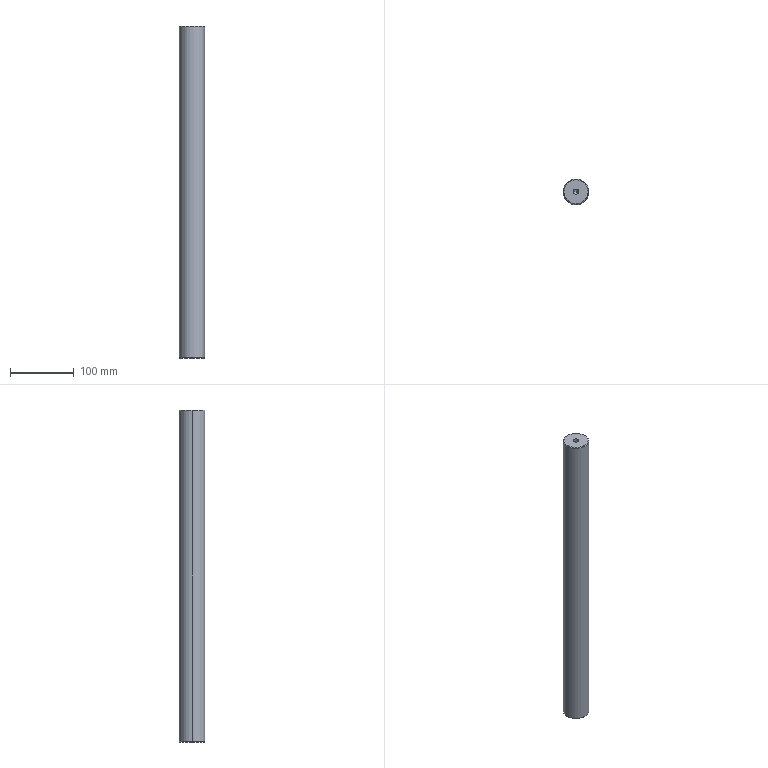Part | SolidWorks | features Chamfer 2, HoleWzd 2, Extrusion 1 | 1 solid | 16 faces | box 40 x 40 x 520 mm | volume 650025 mm3 | cone 8 | cylinder 6 | plane 2 | commonest cylinder face diameters 8.5 x4 40 x2
STEP:
#1=CARTESIAN_POINT('',(-4.25,0.,495.5));
#2=VERTEX_POINT('',#1);
#3=CARTESIAN_POINT('',(4.25,0.,495.5));
#4=VERTEX_POINT('',#3);
#5=CARTESIAN_POINT('',(0.,0.,495.5));
#6=DIRECTION('',(0.,0.,1.));
#7=DIRECTION('',(1.,0.,0.));
#8=AXIS2_PLACEMENT_3D('',#5,#6,#7);
#9=CIRCLE('',#8,4.25);
#10=EDGE_CURVE('',#2,#4,#9,.T.);
#11=ORIENTED_EDGE('',*,*,#10,.F.);
#12=CARTESIAN_POINT('',(-4.25,0.,520.));
#13=VERTEX_POINT('',#12);
#14=CARTESIAN_POINT('',(-4.25,0.,520.));
#15=DIRECTION('',(0.,0.,1.));
#16=VECTOR('',#15,1000.);
#17=LINE('',#14,#16);
#18=EDGE_CURVE('',#2,#13,#17,.T.);
#19=ORIENTED_EDGE('',*,*,#18,.T.);
#20=CARTESIAN_POINT('',(4.25,0.,520.));
#21=VERTEX_POINT('',#20);
#22=CARTESIAN_POINT('',(0.,0.,520.));
#23=DIRECTION('',(0.,0.,1.));
#24=DIRECTION('',(1.,0.,0.));
#25=AXIS2_PLACEMENT_3D('',#22,#23,#24);
#26=CIRCLE('',#25,4.25);
#27=EDGE_CURVE('',#13,#21,#26,.T.);
#28=ORIENTED_EDGE('',*,*,#27,.T.);
#29=CARTESIAN_POINT('',(4.25,0.,520.));
#30=DIRECTION('',(0.,0.,1.));
#31=VECTOR('',#30,1000.);
#32=LINE('',#29,#31);
#33=EDGE_CURVE('',#4,#21,#32,.T.);
#34=ORIENTED_EDGE('',*,*,#33,.F.);
#35=EDGE_LOOP('',(#11,#19,#28,#34));
#36=FACE_OUTER_BOUND('',#35,.T.);
#37=CARTESIAN_POINT('',(0.,0.,520.));
#38=DIRECTION('',(0.,0.,1.));
#39=DIRECTION('',(1.,0.,0.));
#40=AXIS2_PLACEMENT_3D('',#37,#38,#39);
#41=CYLINDRICAL_SURFACE('',#40,4.25);
#42=ADVANCED_FACE('',(#36),#41,.F.);
#43=CARTESIAN_POINT('',(0.,0.,492.946));
#44=VERTEX_POINT('',#43);
#45=CARTESIAN_POINT('',(4.25,0.,495.5));
#46=DIRECTION('',(0.8572,0.,0.515));
#47=VECTOR('',#46,1000.);
#48=LINE('',#45,#47);
#49=EDGE_CURVE('',#44,#4,#48,.T.);
#50=ORIENTED_EDGE('',*,*,#49,.F.);
#51=CARTESIAN_POINT('',(-4.25,0.,495.5));
#52=DIRECTION('',(-0.8572,0.,0.515));
#53=VECTOR('',#52,1000.);
#54=LINE('',#51,#53);
#55=EDGE_CURVE('',#44,#2,#54,.T.);
#56=ORIENTED_EDGE('',*,*,#55,.T.);
#57=ORIENTED_EDGE('',*,*,#10,.T.);
#58=EDGE_LOOP('',(#50,#56,#57));
#59=FACE_OUTER_BOUND('',#58,.T.);
#60=CARTESIAN_POINT('',(0.,0.,495.5));
#61=DIRECTION('',(0.,0.,1.));
#62=DIRECTION('',(1.,0.,0.));
#63=AXIS2_PLACEMENT_3D('',#60,#61,#62);
#64=CONICAL_SURFACE('',#63,4.25,1.03);
#65=ADVANCED_FACE('',(#59),#64,.F.);
#66=CARTESIAN_POINT('',(-19.,0.,0.));
#67=VERTEX_POINT('',#66);
#68=CARTESIAN_POINT('',(19.,0.,0.));
#69=VERTEX_POINT('',#68);
#70=CARTESIAN_POINT('',(0.,0.,0.));
#71=DIRECTION('',(0.,0.,-1.));
#72=DIRECTION('',(1.,0.,0.));
#73=AXIS2_PLACEMENT_3D('',#70,#71,#72);
#74=CIRCLE('',#73,19.);
#75=EDGE_CURVE('',#67,#69,#74,.T.);
#76=ORIENTED_EDGE('',*,*,#75,.F.);
#77=CARTESIAN_POINT('',(-20.,0.,1.));
#78=VERTEX_POINT('',#77);
#79=CARTESIAN_POINT('',(-20.,0.,1.));
#80=DIRECTION('',(-0.7071,0.,0.7071));
#81=VECTOR('',#80,1000.);
#82=LINE('',#79,#81);
#83=EDGE_CURVE('',#67,#78,#82,.T.);
#84=ORIENTED_EDGE('',*,*,#83,.T.);
#85=CARTESIAN_POINT('',(20.,0.,1.));
#86=VERTEX_POINT('',#85);
#87=CARTESIAN_POINT('',(0.,0.,1.));
#88=DIRECTION('',(0.,0.,1.));
#89=DIRECTION('',(1.,0.,0.));
#90=AXIS2_PLACEMENT_3D('',#87,#88,#89);
#91=CIRCLE('',#90,20.);
#92=EDGE_CURVE('',#86,#78,#91,.T.);
#93=ORIENTED_EDGE('',*,*,#92,.F.);
#94=CARTESIAN_POINT('',(20.,0.,1.));
#95=DIRECTION('',(0.7071,0.,0.7071));
#96=VECTOR('',#95,1000.);
#97=LINE('',#94,#96);
#98=EDGE_CURVE('',#69,#86,#97,.T.);
#99=ORIENTED_EDGE('',*,*,#98,.F.);
#100=EDGE_LOOP('',(#76,#84,#93,#99));
#101=FACE_OUTER_BOUND('',#100,.T.);
#102=CARTESIAN_POINT('',(0.,0.,1.));
#103=DIRECTION('',(0.,0.,1.));
#104=DIRECTION('',(1.,0.,0.));
#105=AXIS2_PLACEMENT_3D('',#102,#103,#104);
#106=CONICAL_SURFACE('',#105,20.,0.7854);
#107=ADVANCED_FACE('',(#101),#106,.T.);
#108=CARTESIAN_POINT('',(19.,0.,520.));
#109=VERTEX_POINT('',#108);
#110=CARTESIAN_POINT('',(-19.,0.,520.));
#111=VERTEX_POINT('',#110);
#112=CARTESIAN_POINT('',(0.,0.,520.));
#113=DIRECTION('',(0.,0.,1.));
#114=DIRECTION('',(1.,0.,0.));
#115=AXIS2_PLACEMENT_3D('',#112,#113,#114);
#116=CIRCLE('',#115,19.);
#117=EDGE_CURVE('',#109,#111,#116,.T.);
#118=ORIENTED_EDGE('',*,*,#117,.F.);
#119=CARTESIAN_POINT('',(20.,0.,519.));
#120=VERTEX_POINT('',#119);
#121=CARTESIAN_POINT('',(19.,0.,520.));
#122=DIRECTION('',(0.7071,0.,-0.7071));
#123=VECTOR('',#122,1000.);
#124=LINE('',#121,#123);
#125=EDGE_CURVE('',#109,#120,#124,.T.);
#126=ORIENTED_EDGE('',*,*,#125,.T.);
#127=CARTESIAN_POINT('',(-20.,0.,519.));
#128=VERTEX_POINT('',#127);
#129=CARTESIAN_POINT('',(0.,0.,519.));
#130=DIRECTION('',(0.,0.,-1.));
#131=DIRECTION('',(1.,0.,0.));
#132=AXIS2_PLACEMENT_3D('',#129,#130,#131);
#133=CIRCLE('',#132,20.);
#134=EDGE_CURVE('',#128,#120,#133,.T.);
#135=ORIENTED_EDGE('',*,*,#134,.F.);
#136=CARTESIAN_POINT('',(-19.,0.,520.));
#137=DIRECTION('',(-0.7071,0.,-0.7071));
#138=VECTOR('',#137,1000.);
#139=LINE('',#136,#138);
#140=EDGE_CURVE('',#111,#128,#139,.T.);
#141=ORIENTED_EDGE('',*,*,#140,.F.);
#142=EDGE_LOOP('',(#118,#126,#135,#141));
#143=FACE_OUTER_BOUND('',#142,.T.);
#144=CARTESIAN_POINT('',(0.,0.,520.));
#145=DIRECTION('',(0.,0.,-1.));
#146=DIRECTION('',(-1.,0.,0.));
#147=AXIS2_PLACEMENT_3D('',#144,#145,#146);
#148=CONICAL_SURFACE('',#147,19.,0.7854);
#149=ADVANCED_FACE('',(#143),#148,.T.);
#150=CARTESIAN_POINT('',(4.25,0.,32.));
#151=VERTEX_POINT('',#150);
#152=CARTESIAN_POINT('',(-4.25,0.,32.));
#153=VERTEX_POINT('',#152);
#154=CARTESIAN_POINT('',(0.,0.,32.));
#155=DIRECTION('',(0.,0.,-1.));
#156=DIRECTION('',(-1.,0.,0.));
#157=AXIS2_PLACEMENT_3D('',#154,#155,#156);
#158=CIRCLE('',#157,4.25);
#159=EDGE_CURVE('',#151,#153,#158,.T.);
#160=ORIENTED_EDGE('',*,*,#159,.F.);
#161=CARTESIAN_POINT('',(4.25,0.,0.));
#162=VERTEX_POINT('',#161);
#163=CARTESIAN_POINT('',(4.25,0.,0.));
#164=DIRECTION('',(0.,0.,-1.));
#165=VECTOR('',#164,1000.);
#166=LINE('',#163,#165);
#167=EDGE_CURVE('',#151,#162,#166,.T.);
#168=ORIENTED_EDGE('',*,*,#167,.T.);
#169=CARTESIAN_POINT('',(-4.25,0.,0.));
#170=VERTEX_POINT('',#169);
#171=CARTESIAN_POINT('',(0.,0.,0.));
#172=DIRECTION('',(0.,0.,-1.));
#173=DIRECTION('',(-1.,0.,0.));
#174=AXIS2_PLACEMENT_3D('',#171,#172,#173);
#175=CIRCLE('',#174,4.25);
#176=EDGE_CURVE('',#162,#170,#175,.T.);
#177=ORIENTED_EDGE('',*,*,#176,.T.);
#178=CARTESIAN_POINT('',(-4.25,0.,0.));
#179=DIRECTION('',(0.,0.,-1.));
#180=VECTOR('',#179,1000.);
#181=LINE('',#178,#180);
#182=EDGE_CURVE('',#153,#170,#181,.T.);
#183=ORIENTED_EDGE('',*,*,#182,.F.);
#184=EDGE_LOOP('',(#160,#168,#177,#183));
#185=FACE_OUTER_BOUND('',#184,.T.);
#186=CARTESIAN_POINT('',(0.,0.,0.));
#187=DIRECTION('',(0.,0.,-1.));
#188=DIRECTION('',(-1.,0.,0.));
#189=AXIS2_PLACEMENT_3D('',#186,#187,#188);
#190=CYLINDRICAL_SURFACE('',#189,4.25);
#191=ADVANCED_FACE('',(#185),#190,.F.);
#192=CARTESIAN_POINT('',(0.,0.,34.554));
#193=VERTEX_POINT('',#192);
#194=CARTESIAN_POINT('',(-4.25,0.,32.));
#195=DIRECTION('',(-0.8572,0.,-0.515));
#196=VECTOR('',#195,1000.);
#197=LINE('',#194,#196);
#198=EDGE_CURVE('',#193,#153,#197,.T.);
#199=ORIENTED_EDGE('',*,*,#198,.F.);
#200=CARTESIAN_POINT('',(4.25,0.,32.));
#201=DIRECTION('',(0.8572,0.,-0.515));
#202=VECTOR('',#201,1000.);
#203=LINE('',#200,#202);
#204=EDGE_CURVE('',#193,#151,#203,.T.);
#205=ORIENTED_EDGE('',*,*,#204,.T.);
#206=ORIENTED_EDGE('',*,*,#159,.T.);
#207=EDGE_LOOP('',(#199,#205,#206));
#208=FACE_OUTER_BOUND('',#207,.T.);
#209=CARTESIAN_POINT('',(0.,0.,32.));
#210=DIRECTION('',(0.,0.,-1.));
#211=DIRECTION('',(-1.,0.,0.));
#212=AXIS2_PLACEMENT_3D('',#209,#210,#211);
#213=CONICAL_SURFACE('',#212,4.25,1.03);
#214=ADVANCED_FACE('',(#208),#213,.F.);
#215=ORIENTED_EDGE('',*,*,#134,.T.);
#216=CARTESIAN_POINT('',(20.,0.,520.));
#217=DIRECTION('',(0.,0.,-1.));
#218=VECTOR('',#217,1000.);
#219=LINE('',#216,#218);
#220=EDGE_CURVE('',#120,#86,#219,.T.);
#221=ORIENTED_EDGE('',*,*,#220,.T.);
#222=ORIENTED_EDGE('',*,*,#92,.T.);
#223=CARTESIAN_POINT('',(-20.,0.,520.));
#224=DIRECTION('',(0.,0.,-1.));
#225=VECTOR('',#224,1000.);
#226=LINE('',#223,#225);
#227=EDGE_CURVE('',#128,#78,#226,.T.);
#228=ORIENTED_EDGE('',*,*,#227,.F.);
#229=EDGE_LOOP('',(#215,#221,#222,#228));
#230=FACE_OUTER_BOUND('',#229,.T.);
#231=CARTESIAN_POINT('',(0.,0.,520.));
#232=DIRECTION('',(0.,0.,-1.));
#233=DIRECTION('',(-1.,0.,0.));
#234=AXIS2_PLACEMENT_3D('',#231,#232,#233);
#235=CYLINDRICAL_SURFACE('',#234,20.);
#236=ADVANCED_FACE('',(#230),#235,.T.);
#237=ORIENTED_EDGE('',*,*,#220,.F.);
#238=CARTESIAN_POINT('',(0.,0.,519.));
#239=DIRECTION('',(0.,0.,-1.));
#240=DIRECTION('',(1.,0.,0.));
#241=AXIS2_PLACEMENT_3D('',#238,#239,#240);
#242=CIRCLE('',#241,20.);
#243=EDGE_CURVE('',#120,#128,#242,.T.);
#244=ORIENTED_EDGE('',*,*,#243,.T.);
#245=ORIENTED_EDGE('',*,*,#227,.T.);
#246=CARTESIAN_POINT('',(0.,0.,1.));
#247=DIRECTION('',(0.,0.,1.));
#248=DIRECTION('',(1.,0.,0.));
#249=AXIS2_PLACEMENT_3D('',#246,#247,#248);
#250=CIRCLE('',#249,20.);
#251=EDGE_CURVE('',#78,#86,#250,.T.);
#252=ORIENTED_EDGE('',*,*,#251,.T.);
#253=EDGE_LOOP('',(#237,#244,#245,#252));
#254=FACE_OUTER_BOUND('',#253,.T.);
#255=CARTESIAN_POINT('',(0.,0.,520.));
#256=DIRECTION('',(0.,0.,-1.));
#257=DIRECTION('',(-1.,0.,0.));
#258=AXIS2_PLACEMENT_3D('',#255,#256,#257);
#259=CYLINDRICAL_SURFACE('',#258,20.);
#260=ADVANCED_FACE('',(#254),#259,.T.);
#261=CARTESIAN_POINT('',(0.,0.,520.));
#262=DIRECTION('',(0.,0.,1.));
#263=DIRECTION('',(1.,0.,0.));
#264=AXIS2_PLACEMENT_3D('',#261,#262,#263);
#265=CIRCLE('',#264,4.25);
#266=EDGE_CURVE('',#21,#13,#265,.T.);
#267=ORIENTED_EDGE('',*,*,#266,.F.);
#268=ORIENTED_EDGE('',*,*,#27,.F.);
#269=EDGE_LOOP('',(#267,#268));
#270=FACE_BOUND('',#269,.T.);
#271=CARTESIAN_POINT('',(0.,0.,520.));
#272=DIRECTION('',(0.,0.,1.));
#273=DIRECTION('',(1.,0.,0.));
#274=AXIS2_PLACEMENT_3D('',#271,#272,#273);
#275=CIRCLE('',#274,19.);
#276=EDGE_CURVE('',#111,#109,#275,.T.);
#277=ORIENTED_EDGE('',*,*,#276,.T.);
#278=ORIENTED_EDGE('',*,*,#117,.T.);
#279=EDGE_LOOP('',(#277,#278));
#280=FACE_OUTER_BOUND('',#279,.T.);
#281=CARTESIAN_POINT('',(0.,0.,520.));
#282=DIRECTION('',(0.,0.,1.));
#283=DIRECTION('',(1.,0.,0.));
#284=AXIS2_PLACEMENT_3D('',#281,#282,#283);
#285=PLANE('',#284);
#286=ADVANCED_FACE('',(#270,#280),#285,.T.);
#287=CARTESIAN_POINT('',(0.,0.,0.));
#288=DIRECTION('',(0.,0.,-1.));
#289=DIRECTION('',(1.,0.,0.));
#290=AXIS2_PLACEMENT_3D('',#287,#288,#289);
#291=CIRCLE('',#290,19.);
#292=EDGE_CURVE('',#69,#67,#291,.T.);
#293=ORIENTED_EDGE('',*,*,#292,.T.);
#294=ORIENTED_EDGE('',*,*,#75,.T.);
#295=EDGE_LOOP('',(#293,#294));
#296=FACE_OUTER_BOUND('',#295,.T.);
#297=CARTESIAN_POINT('',(0.,0.,0.));
#298=DIRECTION('',(0.,0.,-1.));
#299=DIRECTION('',(-1.,0.,0.));
#300=AXIS2_PLACEMENT_3D('',#297,#298,#299);
#301=CIRCLE('',#300,4.25);
#302=EDGE_CURVE('',#170,#162,#301,.T.);
#303=ORIENTED_EDGE('',*,*,#302,.F.);
#304=ORIENTED_EDGE('',*,*,#176,.F.);
#305=EDGE_LOOP('',(#303,#304));
#306=FACE_BOUND('',#305,.T.);
#307=CARTESIAN_POINT('',(0.,0.,0.));
#308=DIRECTION('',(0.,0.,1.));
#309=DIRECTION('',(1.,0.,0.));
#310=AXIS2_PLACEMENT_3D('',#307,#308,#309);
#311=PLANE('',#310);
#312=ADVANCED_FACE('',(#296,#306),#311,.F.);
#313=ORIENTED_EDGE('',*,*,#204,.F.);
#314=ORIENTED_EDGE('',*,*,#198,.T.);
#315=CARTESIAN_POINT('',(0.,0.,32.));
#316=DIRECTION('',(0.,0.,-1.));
#317=DIRECTION('',(-1.,0.,0.));
#318=AXIS2_PLACEMENT_3D('',#315,#316,#317);
#319=CIRCLE('',#318,4.25);
#320=EDGE_CURVE('',#153,#151,#319,.T.);
#321=ORIENTED_EDGE('',*,*,#320,.T.);
#322=EDGE_LOOP('',(#313,#314,#321));
#323=FACE_OUTER_BOUND('',#322,.T.);
#324=CARTESIAN_POINT('',(0.,0.,32.));
#325=DIRECTION('',(0.,0.,-1.));
#326=DIRECTION('',(-1.,0.,0.));
#327=AXIS2_PLACEMENT_3D('',#324,#325,#326);
#328=CONICAL_SURFACE('',#327,4.25,1.03);
#329=ADVANCED_FACE('',(#323),#328,.F.);
#330=ORIENTED_EDGE('',*,*,#167,.F.);
#331=ORIENTED_EDGE('',*,*,#320,.F.);
#332=ORIENTED_EDGE('',*,*,#182,.T.);
#333=ORIENTED_EDGE('',*,*,#302,.T.);
#334=EDGE_LOOP('',(#330,#331,#332,#333));
#335=FACE_OUTER_BOUND('',#334,.T.);
#336=CARTESIAN_POINT('',(0.,0.,0.));
#337=DIRECTION('',(0.,0.,-1.));
#338=DIRECTION('',(-1.,0.,0.));
#339=AXIS2_PLACEMENT_3D('',#336,#337,#338);
#340=CYLINDRICAL_SURFACE('',#339,4.25);
#341=ADVANCED_FACE('',(#335),#340,.F.);
#342=ORIENTED_EDGE('',*,*,#125,.F.);
#343=ORIENTED_EDGE('',*,*,#276,.F.);
#344=ORIENTED_EDGE('',*,*,#140,.T.);
#345=ORIENTED_EDGE('',*,*,#243,.F.);
#346=EDGE_LOOP('',(#342,#343,#344,#345));
#347=FACE_OUTER_BOUND('',#346,.T.);
#348=CARTESIAN_POINT('',(0.,0.,520.));
#349=DIRECTION('',(0.,0.,-1.));
#350=DIRECTION('',(-1.,0.,0.));
#351=AXIS2_PLACEMENT_3D('',#348,#349,#350);
#352=CONICAL_SURFACE('',#351,19.,0.7854);
#353=ADVANCED_FACE('',(#347),#352,.T.);
#354=ORIENTED_EDGE('',*,*,#83,.F.);
#355=ORIENTED_EDGE('',*,*,#292,.F.);
#356=ORIENTED_EDGE('',*,*,#98,.T.);
#357=ORIENTED_EDGE('',*,*,#251,.F.);
#358=EDGE_LOOP('',(#354,#355,#356,#357));
#359=FACE_OUTER_BOUND('',#358,.T.);
#360=CARTESIAN_POINT('',(0.,0.,1.));
#361=DIRECTION('',(0.,0.,1.));
#362=DIRECTION('',(1.,0.,0.));
#363=AXIS2_PLACEMENT_3D('',#360,#361,#362);
#364=CONICAL_SURFACE('',#363,20.,0.7854);
#365=ADVANCED_FACE('',(#359),#364,.T.);
#366=ORIENTED_EDGE('',*,*,#55,.F.);
#367=ORIENTED_EDGE('',*,*,#49,.T.);
#368=CARTESIAN_POINT('',(0.,0.,495.5));
#369=DIRECTION('',(0.,0.,1.));
#370=DIRECTION('',(1.,0.,0.));
#371=AXIS2_PLACEMENT_3D('',#368,#369,#370);
#372=CIRCLE('',#371,4.25);
#373=EDGE_CURVE('',#4,#2,#372,.T.);
#374=ORIENTED_EDGE('',*,*,#373,.T.);
#375=EDGE_LOOP('',(#366,#367,#374));
#376=FACE_OUTER_BOUND('',#375,.T.);
#377=CARTESIAN_POINT('',(0.,0.,495.5));
#378=DIRECTION('',(0.,0.,1.));
#379=DIRECTION('',(1.,0.,0.));
#380=AXIS2_PLACEMENT_3D('',#377,#378,#379);
#381=CONICAL_SURFACE('',#380,4.25,1.03);
#382=ADVANCED_FACE('',(#376),#381,.F.);
#383=ORIENTED_EDGE('',*,*,#18,.F.);
#384=ORIENTED_EDGE('',*,*,#373,.F.);
#385=ORIENTED_EDGE('',*,*,#33,.T.);
#386=ORIENTED_EDGE('',*,*,#266,.T.);
#387=EDGE_LOOP('',(#383,#384,#385,#386));
#388=FACE_OUTER_BOUND('',#387,.T.);
#389=CARTESIAN_POINT('',(0.,0.,520.));
#390=DIRECTION('',(0.,0.,1.));
#391=DIRECTION('',(1.,0.,0.));
#392=AXIS2_PLACEMENT_3D('',#389,#390,#391);
#393=CYLINDRICAL_SURFACE('',#392,4.25);
#394=ADVANCED_FACE('',(#388),#393,.F.);
#395=CLOSED_SHELL('',(#42,#65,#107,#149,#191,#214,#236,#260,#286,#312,#329,#341,#353,#365,#382,#394));
#396=MANIFOLD_SOLID_BREP('',#395);
#397=CARTESIAN_POINT('',(0.,0.,0.));
#398=DIRECTION('',(0.,0.,1.));
#399=DIRECTION('',(1.,0.,0.));
#400=AXIS2_PLACEMENT_3D('',#397,#398,#399);
#401=(LENGTH_UNIT()NAMED_UNIT(*)SI_UNIT(.MILLI.,.METRE.));
#402=UNCERTAINTY_MEASURE_WITH_UNIT(LENGTH_MEASURE(0.00001),#401,'','');
#403=(NAMED_UNIT(*)PLANE_ANGLE_UNIT()SI_UNIT($,.RADIAN.));
#404=(NAMED_UNIT(*)SI_UNIT($,.STERADIAN.)SOLID_ANGLE_UNIT());
#405=(GEOMETRIC_REPRESENTATION_CONTEXT(3)GLOBAL_UNCERTAINTY_ASSIGNED_CONTEXT((#402))GLOBAL_UNIT_ASSIGNED_CONTEXT((#401,#403,#404))REPRESENTATION_CONTEXT('',''));
#406=ADVANCED_BREP_SHAPE_REPRESENTATION('',(#396,#400),#405);